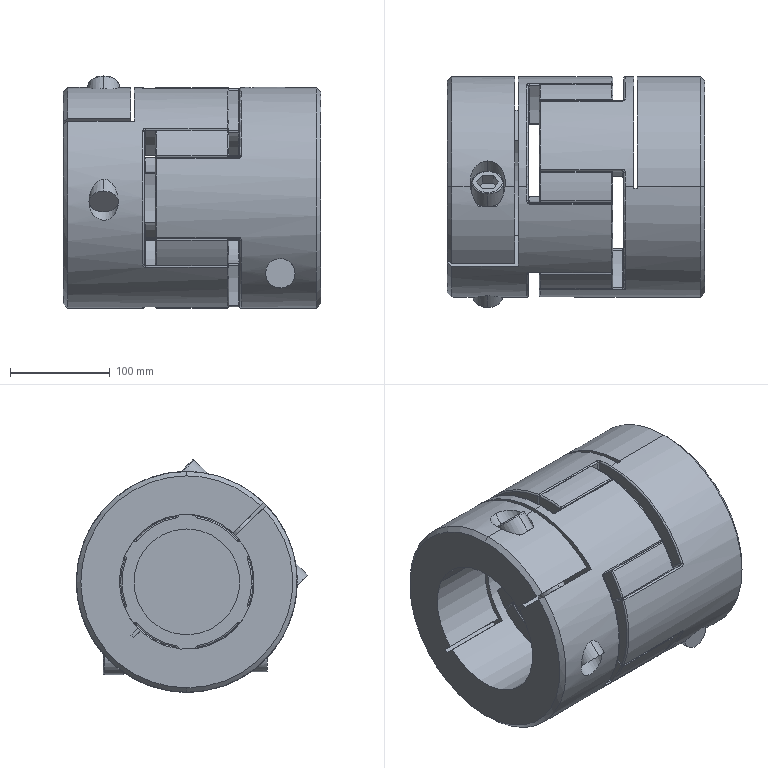Part | NX | features SCALE 4, BREP 3, LINKED_BODY 2, SUBTRACT 2 | 3 solids | 410 faces | box 257.704 x 231.242 x 232.662 mm | volume 6465109 mm3 | torus 142 | cylinder 134 | plane 59 | sphere 58 | spline 12 | cone 5 | commonest cylinder face diameters 2.945 x58 132.534 x36 220.889 x13 29.452 x10 106.027 x4 35.342 x3